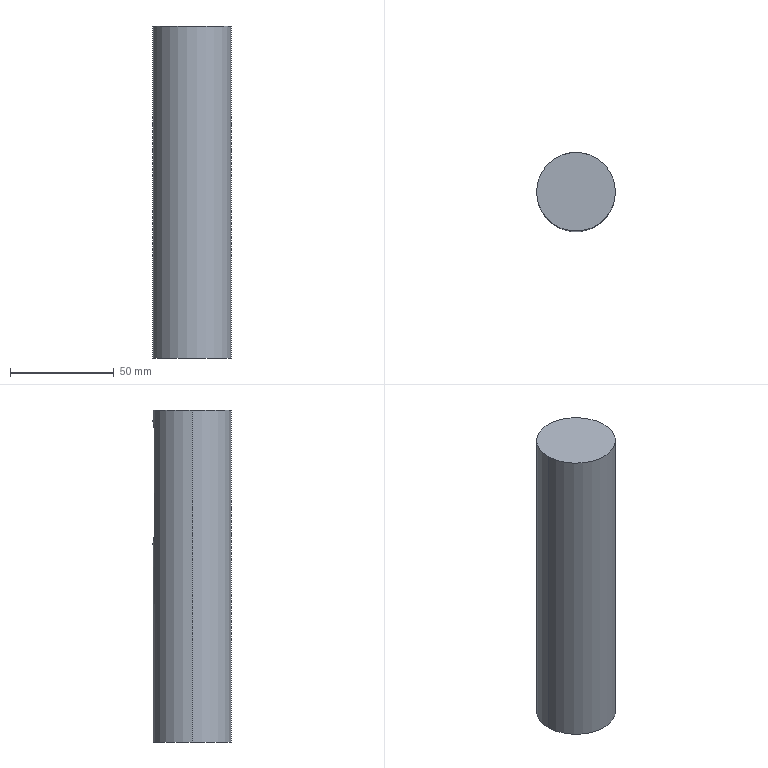Part | SolidWorks | features Extrusion 1, ICE 1 | 1 solid | 10 faces | box 38 x 38 x 160 mm | volume 178690 mm3 | cylinder 5 | plane 5 | commonest cylinder face diameters 10 x3 38 x2
STEP:
#1=CARTESIAN_POINT('',(5.,18.33,100.));
#2=VERTEX_POINT('',#1);
#3=CARTESIAN_POINT('',(0.,19.,95.));
#4=VERTEX_POINT('',#3);
#5=CARTESIAN_POINT('',(5.,18.33,100.));
#6=CARTESIAN_POINT('',(5.,18.33,99.668));
#7=CARTESIAN_POINT('',(4.967,18.339,99.342));
#8=CARTESIAN_POINT('',(4.839,18.374,98.701));
#9=CARTESIAN_POINT('',(4.742,18.399,98.382));
#10=CARTESIAN_POINT('',(4.491,18.462,97.777));
#11=CARTESIAN_POINT('',(4.337,18.499,97.491));
#12=CARTESIAN_POINT('',(3.974,18.581,96.948));
#13=CARTESIAN_POINT('',(3.764,18.625,96.692));
#14=CARTESIAN_POINT('',(3.304,18.712,96.233));
#15=CARTESIAN_POINT('',(3.053,18.755,96.027));
#16=CARTESIAN_POINT('',(2.507,18.836,95.661));
#17=CARTESIAN_POINT('',(2.218,18.872,95.507));
#18=CARTESIAN_POINT('',(1.767,18.918,95.32));
#19=CARTESIAN_POINT('',(1.613,18.932,95.265));
#20=CARTESIAN_POINT('',(1.299,18.956,95.169));
#21=CARTESIAN_POINT('',(1.138,18.967,95.128));
#22=CARTESIAN_POINT('',(0.6534,18.992,95.032));
#23=CARTESIAN_POINT('',(0.3279,19.,95.));
#24=CARTESIAN_POINT('',(0.,19.,95.));
#25=B_SPLINE_CURVE_WITH_KNOTS('',3,(#5,#6,#7,#8,#9,#10,#11,#12,#13,#14,#15,#16,#17,#18,#19,#20,#21,#22,#23,#24),.UNSPECIFIED.,.F.,.F.,(4,2,2,2,2,2,2,2,2,4),(0.,0.0009816,0.001963,0.002945,0.003926,0.004908,0.00589,0.00638,0.006871,0.007853),.UNSPECIFIED.);
#26=EDGE_CURVE('',#2,#4,#25,.T.);
#27=ORIENTED_EDGE('',*,*,#26,.T.);
#28=CARTESIAN_POINT('',(0.,14.,95.));
#29=VERTEX_POINT('',#28);
#30=CARTESIAN_POINT('',(0.,19.,95.));
#31=DIRECTION('',(0.,-1.,0.));
#32=VECTOR('',#31,1000.);
#33=LINE('',#30,#32);
#34=EDGE_CURVE('',#4,#29,#33,.T.);
#35=ORIENTED_EDGE('',*,*,#34,.T.);
#36=CARTESIAN_POINT('',(5.,14.,100.));
#37=VERTEX_POINT('',#36);
#38=CARTESIAN_POINT('',(0.,14.,100.));
#39=DIRECTION('',(0.,1.,0.));
#40=DIRECTION('',(0.,0.,1.));
#41=AXIS2_PLACEMENT_3D('',#38,#39,#40);
#42=CIRCLE('',#41,5.);
#43=EDGE_CURVE('',#37,#29,#42,.T.);
#44=ORIENTED_EDGE('',*,*,#43,.F.);
#45=CARTESIAN_POINT('',(5.,19.,100.));
#46=DIRECTION('',(0.,-1.,0.));
#47=VECTOR('',#46,1000.);
#48=LINE('',#45,#47);
#49=EDGE_CURVE('',#2,#37,#48,.T.);
#50=ORIENTED_EDGE('',*,*,#49,.F.);
#51=EDGE_LOOP('',(#27,#35,#44,#50));
#52=FACE_OUTER_BOUND('',#51,.T.);
#53=CARTESIAN_POINT('',(0.,19.,100.));
#54=DIRECTION('',(0.,-1.,0.));
#55=DIRECTION('',(0.,0.,-1.));
#56=AXIS2_PLACEMENT_3D('',#53,#54,#55);
#57=CYLINDRICAL_SURFACE('',#56,5.);
#58=ADVANCED_FACE('',(#52),#57,.F.);
#59=ORIENTED_EDGE('',*,*,#26,.F.);
#60=CARTESIAN_POINT('',(5.,18.33,150.));
#61=VERTEX_POINT('',#60);
#62=CARTESIAN_POINT('',(5.,18.33,160.));
#63=DIRECTION('',(0.,0.,-1.));
#64=VECTOR('',#63,1000.);
#65=LINE('',#62,#64);
#66=EDGE_CURVE('',#61,#2,#65,.T.);
#67=ORIENTED_EDGE('',*,*,#66,.F.);
#68=CARTESIAN_POINT('',(-5.,18.33,150.));
#69=VERTEX_POINT('',#68);
#70=CARTESIAN_POINT('',(-5.,18.33,150.));
#71=CARTESIAN_POINT('',(-5.,18.33,150.332));
#72=CARTESIAN_POINT('',(-4.967,18.339,150.658));
#73=CARTESIAN_POINT('',(-4.839,18.373,151.299));
#74=CARTESIAN_POINT('',(-4.743,18.399,151.617));
#75=CARTESIAN_POINT('',(-4.491,18.462,152.222));
#76=CARTESIAN_POINT('',(-4.338,18.499,152.508));
#77=CARTESIAN_POINT('',(-3.975,18.58,153.05));
#78=CARTESIAN_POINT('',(-3.765,18.625,153.306));
#79=CARTESIAN_POINT('',(-3.306,18.712,153.765));
#80=CARTESIAN_POINT('',(-3.056,18.755,153.971));
#81=CARTESIAN_POINT('',(-2.51,18.836,154.337));
#82=CARTESIAN_POINT('',(-2.221,18.872,154.491));
#83=CARTESIAN_POINT('',(-1.77,18.918,154.679));
#84=CARTESIAN_POINT('',(-1.617,18.932,154.734));
#85=CARTESIAN_POINT('',(-1.303,18.956,154.83));
#86=CARTESIAN_POINT('',(-1.142,18.966,154.871));
#87=CARTESIAN_POINT('',(-0.6576,18.991,154.968));
#88=CARTESIAN_POINT('',(-0.3322,19.,155.));
#89=CARTESIAN_POINT('',(0.3231,19.,155.));
#90=CARTESIAN_POINT('',(0.656,18.991,154.968));
#91=CARTESIAN_POINT('',(1.298,18.958,154.84));
#92=CARTESIAN_POINT('',(1.611,18.934,154.745));
#93=CARTESIAN_POINT('',(2.218,18.873,154.493));
#94=CARTESIAN_POINT('',(2.508,18.836,154.337));
#95=CARTESIAN_POINT('',(3.049,18.756,153.976));
#96=CARTESIAN_POINT('',(3.303,18.712,153.768));
#97=CARTESIAN_POINT('',(3.766,18.625,153.306));
#98=CARTESIAN_POINT('',(3.971,18.581,153.055));
#99=CARTESIAN_POINT('',(4.334,18.5,152.515));
#100=CARTESIAN_POINT('',(4.491,18.462,152.222));
#101=CARTESIAN_POINT('',(4.742,18.399,151.619));
#102=CARTESIAN_POINT('',(4.837,18.374,151.308));
#103=CARTESIAN_POINT('',(4.967,18.34,150.664));
#104=CARTESIAN_POINT('',(5.,18.33,150.332));
#105=CARTESIAN_POINT('',(5.,18.33,150.));
#106=B_SPLINE_CURVE_WITH_KNOTS('',3,(#70,#71,#72,#73,#74,#75,#76,#77,#78,#79,#80,#81,#82,#83,#84,#85,#86,#87,#88,#89,#90,#91,#92,#93,#94,#95,#96,#97,#98,#99,#100,#101,#102,#103,#104,#105),.UNSPECIFIED.,.F.,.F.,(4,2,2,2,2,2,2,2,2,2,2,2,2,2,2,2,2,4),(0.,0.000981,0.001962,0.002943,0.003924,0.004905,0.005886,0.006377,0.006867,0.007848,0.008829,0.00981,0.01079,0.01177,0.01275,0.01373,0.01472,0.0157),.UNSPECIFIED.);
#107=EDGE_CURVE('',#69,#61,#106,.T.);
#108=ORIENTED_EDGE('',*,*,#107,.F.);
#109=CARTESIAN_POINT('',(-5.,18.33,100.));
#110=VERTEX_POINT('',#109);
#111=CARTESIAN_POINT('',(-5.,18.33,160.));
#112=DIRECTION('',(0.,0.,1.));
#113=VECTOR('',#112,1000.);
#114=LINE('',#111,#113);
#115=EDGE_CURVE('',#110,#69,#114,.T.);
#116=ORIENTED_EDGE('',*,*,#115,.F.);
#117=CARTESIAN_POINT('',(0.,19.,95.));
#118=CARTESIAN_POINT('',(-0.3275,19.,95.));
#119=CARTESIAN_POINT('',(-0.6602,18.991,95.033));
#120=CARTESIAN_POINT('',(-1.302,18.958,95.161));
#121=CARTESIAN_POINT('',(-1.614,18.934,95.256));
#122=CARTESIAN_POINT('',(-2.221,18.872,95.508));
#123=CARTESIAN_POINT('',(-2.511,18.835,95.664));
#124=CARTESIAN_POINT('',(-3.051,18.755,96.025));
#125=CARTESIAN_POINT('',(-3.305,18.712,96.233));
#126=CARTESIAN_POINT('',(-3.767,18.624,96.696));
#127=CARTESIAN_POINT('',(-3.973,18.581,96.947));
#128=CARTESIAN_POINT('',(-4.334,18.5,97.486));
#129=CARTESIAN_POINT('',(-4.491,18.462,97.779));
#130=CARTESIAN_POINT('',(-4.742,18.399,98.381));
#131=CARTESIAN_POINT('',(-4.837,18.374,98.693));
#132=CARTESIAN_POINT('',(-4.967,18.339,99.336));
#133=CARTESIAN_POINT('',(-5.,18.33,99.668));
#134=CARTESIAN_POINT('',(-5.,18.33,100.));
#135=B_SPLINE_CURVE_WITH_KNOTS('',3,(#117,#118,#119,#120,#121,#122,#123,#124,#125,#126,#127,#128,#129,#130,#131,#132,#133,#134),.UNSPECIFIED.,.F.,.F.,(4,2,2,2,2,2,2,2,4),(0.007853,0.008833,0.009814,0.01079,0.01177,0.01276,0.01374,0.01472,0.0157),.UNSPECIFIED.);
#136=EDGE_CURVE('',#4,#110,#135,.T.);
#137=ORIENTED_EDGE('',*,*,#136,.F.);
#138=EDGE_LOOP('',(#59,#67,#108,#116,#137));
#139=FACE_BOUND('',#138,.T.);
#140=CARTESIAN_POINT('',(19.,0.,160.));
#141=VERTEX_POINT('',#140);
#142=CARTESIAN_POINT('',(-19.,0.,160.));
#143=VERTEX_POINT('',#142);
#144=CARTESIAN_POINT('',(0.,0.,160.));
#145=DIRECTION('',(0.,0.,1.));
#146=DIRECTION('',(1.,0.,0.));
#147=AXIS2_PLACEMENT_3D('',#144,#145,#146);
#148=CIRCLE('',#147,19.);
#149=EDGE_CURVE('',#141,#143,#148,.T.);
#150=ORIENTED_EDGE('',*,*,#149,.F.);
#151=CARTESIAN_POINT('',(19.,0.,0.));
#152=VERTEX_POINT('',#151);
#153=CARTESIAN_POINT('',(19.,0.,160.));
#154=DIRECTION('',(0.,0.,-1.));
#155=VECTOR('',#154,1000.);
#156=LINE('',#153,#155);
#157=EDGE_CURVE('',#141,#152,#156,.T.);
#158=ORIENTED_EDGE('',*,*,#157,.T.);
#159=CARTESIAN_POINT('',(-19.,0.,0.));
#160=VERTEX_POINT('',#159);
#161=CARTESIAN_POINT('',(0.,0.,0.));
#162=DIRECTION('',(0.,0.,1.));
#163=DIRECTION('',(1.,0.,0.));
#164=AXIS2_PLACEMENT_3D('',#161,#162,#163);
#165=CIRCLE('',#164,19.);
#166=EDGE_CURVE('',#152,#160,#165,.T.);
#167=ORIENTED_EDGE('',*,*,#166,.T.);
#168=CARTESIAN_POINT('',(-19.,0.,160.));
#169=DIRECTION('',(0.,0.,-1.));
#170=VECTOR('',#169,1000.);
#171=LINE('',#168,#170);
#172=EDGE_CURVE('',#143,#160,#171,.T.);
#173=ORIENTED_EDGE('',*,*,#172,.F.);
#174=EDGE_LOOP('',(#150,#158,#167,#173));
#175=FACE_OUTER_BOUND('',#174,.T.);
#176=CARTESIAN_POINT('',(0.,0.,160.));
#177=DIRECTION('',(0.,0.,-1.));
#178=DIRECTION('',(-1.,0.,0.));
#179=AXIS2_PLACEMENT_3D('',#176,#177,#178);
#180=CYLINDRICAL_SURFACE('',#179,19.);
#181=ADVANCED_FACE('',(#139,#175),#180,.T.);
#182=ORIENTED_EDGE('',*,*,#157,.F.);
#183=CARTESIAN_POINT('',(0.,0.,160.));
#184=DIRECTION('',(0.,0.,1.));
#185=DIRECTION('',(1.,0.,0.));
#186=AXIS2_PLACEMENT_3D('',#183,#184,#185);
#187=CIRCLE('',#186,19.);
#188=EDGE_CURVE('',#143,#141,#187,.T.);
#189=ORIENTED_EDGE('',*,*,#188,.F.);
#190=ORIENTED_EDGE('',*,*,#172,.T.);
#191=CARTESIAN_POINT('',(0.,0.,0.));
#192=DIRECTION('',(0.,0.,1.));
#193=DIRECTION('',(1.,0.,0.));
#194=AXIS2_PLACEMENT_3D('',#191,#192,#193);
#195=CIRCLE('',#194,19.);
#196=EDGE_CURVE('',#160,#152,#195,.T.);
#197=ORIENTED_EDGE('',*,*,#196,.T.);
#198=EDGE_LOOP('',(#182,#189,#190,#197));
#199=FACE_OUTER_BOUND('',#198,.T.);
#200=CARTESIAN_POINT('',(0.,0.,160.));
#201=DIRECTION('',(0.,0.,-1.));
#202=DIRECTION('',(-1.,0.,0.));
#203=AXIS2_PLACEMENT_3D('',#200,#201,#202);
#204=CYLINDRICAL_SURFACE('',#203,19.);
#205=ADVANCED_FACE('',(#199),#204,.T.);
#206=ORIENTED_EDGE('',*,*,#188,.T.);
#207=ORIENTED_EDGE('',*,*,#149,.T.);
#208=EDGE_LOOP('',(#206,#207));
#209=FACE_OUTER_BOUND('',#208,.T.);
#210=CARTESIAN_POINT('',(0.,0.,160.));
#211=DIRECTION('',(0.,0.,1.));
#212=DIRECTION('',(1.,0.,0.));
#213=AXIS2_PLACEMENT_3D('',#210,#211,#212);
#214=PLANE('',#213);
#215=ADVANCED_FACE('',(#209),#214,.T.);
#216=ORIENTED_EDGE('',*,*,#196,.F.);
#217=ORIENTED_EDGE('',*,*,#166,.F.);
#218=EDGE_LOOP('',(#216,#217));
#219=FACE_OUTER_BOUND('',#218,.T.);
#220=CARTESIAN_POINT('',(0.,0.,0.));
#221=DIRECTION('',(0.,0.,1.));
#222=DIRECTION('',(1.,0.,0.));
#223=AXIS2_PLACEMENT_3D('',#220,#221,#222);
#224=PLANE('',#223);
#225=ADVANCED_FACE('',(#219),#224,.F.);
#226=CARTESIAN_POINT('',(-5.,14.,150.));
#227=VERTEX_POINT('',#226);
#228=CARTESIAN_POINT('',(-5.,19.,150.));
#229=DIRECTION('',(0.,-1.,0.));
#230=VECTOR('',#229,1000.);
#231=LINE('',#228,#230);
#232=EDGE_CURVE('',#69,#227,#231,.T.);
#233=ORIENTED_EDGE('',*,*,#232,.F.);
#234=ORIENTED_EDGE('',*,*,#107,.T.);
#235=CARTESIAN_POINT('',(5.,14.,150.));
#236=VERTEX_POINT('',#235);
#237=CARTESIAN_POINT('',(5.,19.,150.));
#238=DIRECTION('',(0.,-1.,0.));
#239=VECTOR('',#238,1000.);
#240=LINE('',#237,#239);
#241=EDGE_CURVE('',#61,#236,#240,.T.);
#242=ORIENTED_EDGE('',*,*,#241,.T.);
#243=CARTESIAN_POINT('',(0.,14.,150.));
#244=DIRECTION('',(0.,1.,0.));
#245=DIRECTION('',(0.,0.,1.));
#246=AXIS2_PLACEMENT_3D('',#243,#244,#245);
#247=CIRCLE('',#246,5.);
#248=EDGE_CURVE('',#227,#236,#247,.T.);
#249=ORIENTED_EDGE('',*,*,#248,.F.);
#250=EDGE_LOOP('',(#233,#234,#242,#249));
#251=FACE_OUTER_BOUND('',#250,.T.);
#252=CARTESIAN_POINT('',(0.,19.,150.));
#253=DIRECTION('',(0.,-1.,0.));
#254=DIRECTION('',(0.,0.,-1.));
#255=AXIS2_PLACEMENT_3D('',#252,#253,#254);
#256=CYLINDRICAL_SURFACE('',#255,5.);
#257=ADVANCED_FACE('',(#251),#256,.F.);
#258=ORIENTED_EDGE('',*,*,#66,.T.);
#259=ORIENTED_EDGE('',*,*,#49,.T.);
#260=CARTESIAN_POINT('',(5.,14.,150.));
#261=DIRECTION('',(0.,0.,-1.));
#262=VECTOR('',#261,1000.);
#263=LINE('',#260,#262);
#264=EDGE_CURVE('',#236,#37,#263,.T.);
#265=ORIENTED_EDGE('',*,*,#264,.F.);
#266=ORIENTED_EDGE('',*,*,#241,.F.);
#267=EDGE_LOOP('',(#258,#259,#265,#266));
#268=FACE_OUTER_BOUND('',#267,.T.);
#269=CARTESIAN_POINT('',(5.,19.,150.));
#270=DIRECTION('',(-1.,0.,0.));
#271=DIRECTION('',(0.,0.,1.));
#272=AXIS2_PLACEMENT_3D('',#269,#270,#271);
#273=PLANE('',#272);
#274=ADVANCED_FACE('',(#268),#273,.T.);
#275=ORIENTED_EDGE('',*,*,#34,.F.);
#276=ORIENTED_EDGE('',*,*,#136,.T.);
#277=CARTESIAN_POINT('',(-5.,14.,100.));
#278=VERTEX_POINT('',#277);
#279=CARTESIAN_POINT('',(-5.,19.,100.));
#280=DIRECTION('',(0.,-1.,0.));
#281=VECTOR('',#280,1000.);
#282=LINE('',#279,#281);
#283=EDGE_CURVE('',#110,#278,#282,.T.);
#284=ORIENTED_EDGE('',*,*,#283,.T.);
#285=CARTESIAN_POINT('',(0.,14.,100.));
#286=DIRECTION('',(0.,1.,0.));
#287=DIRECTION('',(0.,0.,1.));
#288=AXIS2_PLACEMENT_3D('',#285,#286,#287);
#289=CIRCLE('',#288,5.);
#290=EDGE_CURVE('',#29,#278,#289,.T.);
#291=ORIENTED_EDGE('',*,*,#290,.F.);
#292=EDGE_LOOP('',(#275,#276,#284,#291));
#293=FACE_OUTER_BOUND('',#292,.T.);
#294=CARTESIAN_POINT('',(0.,19.,100.));
#295=DIRECTION('',(0.,-1.,0.));
#296=DIRECTION('',(0.,0.,-1.));
#297=AXIS2_PLACEMENT_3D('',#294,#295,#296);
#298=CYLINDRICAL_SURFACE('',#297,5.);
#299=ADVANCED_FACE('',(#293),#298,.F.);
#300=ORIENTED_EDGE('',*,*,#115,.T.);
#301=ORIENTED_EDGE('',*,*,#232,.T.);
#302=CARTESIAN_POINT('',(-5.,14.,150.));
#303=DIRECTION('',(0.,0.,1.));
#304=VECTOR('',#303,1000.);
#305=LINE('',#302,#304);
#306=EDGE_CURVE('',#278,#227,#305,.T.);
#307=ORIENTED_EDGE('',*,*,#306,.F.);
#308=ORIENTED_EDGE('',*,*,#283,.F.);
#309=EDGE_LOOP('',(#300,#301,#307,#308));
#310=FACE_OUTER_BOUND('',#309,.T.);
#311=CARTESIAN_POINT('',(-5.,19.,150.));
#312=DIRECTION('',(1.,0.,0.));
#313=DIRECTION('',(0.,0.,-1.));
#314=AXIS2_PLACEMENT_3D('',#311,#312,#313);
#315=PLANE('',#314);
#316=ADVANCED_FACE('',(#310),#315,.T.);
#317=ORIENTED_EDGE('',*,*,#248,.T.);
#318=ORIENTED_EDGE('',*,*,#264,.T.);
#319=ORIENTED_EDGE('',*,*,#43,.T.);
#320=ORIENTED_EDGE('',*,*,#290,.T.);
#321=ORIENTED_EDGE('',*,*,#306,.T.);
#322=EDGE_LOOP('',(#317,#318,#319,#320,#321));
#323=FACE_OUTER_BOUND('',#322,.T.);
#324=CARTESIAN_POINT('',(0.,14.,150.));
#325=DIRECTION('',(0.,1.,0.));
#326=DIRECTION('',(0.,0.,1.));
#327=AXIS2_PLACEMENT_3D('',#324,#325,#326);
#328=PLANE('',#327);
#329=ADVANCED_FACE('',(#323),#328,.T.);
#330=CLOSED_SHELL('',(#58,#181,#205,#215,#225,#257,#274,#299,#316,#329));
#331=MANIFOLD_SOLID_BREP('',#330);
#332=CARTESIAN_POINT('',(0.,0.,0.));
#333=DIRECTION('',(0.,0.,1.));
#334=DIRECTION('',(1.,0.,0.));
#335=AXIS2_PLACEMENT_3D('',#332,#333,#334);
#336=(LENGTH_UNIT()NAMED_UNIT(*)SI_UNIT(.MILLI.,.METRE.));
#337=UNCERTAINTY_MEASURE_WITH_UNIT(LENGTH_MEASURE(0.00001),#336,'','');
#338=(NAMED_UNIT(*)PLANE_ANGLE_UNIT()SI_UNIT($,.RADIAN.));
#339=(NAMED_UNIT(*)SI_UNIT($,.STERADIAN.)SOLID_ANGLE_UNIT());
#340=(GEOMETRIC_REPRESENTATION_CONTEXT(3)GLOBAL_UNCERTAINTY_ASSIGNED_CONTEXT((#337))GLOBAL_UNIT_ASSIGNED_CONTEXT((#336,#338,#339))REPRESENTATION_CONTEXT('',''));
#341=ADVANCED_BREP_SHAPE_REPRESENTATION('',(#331,#335),#340);